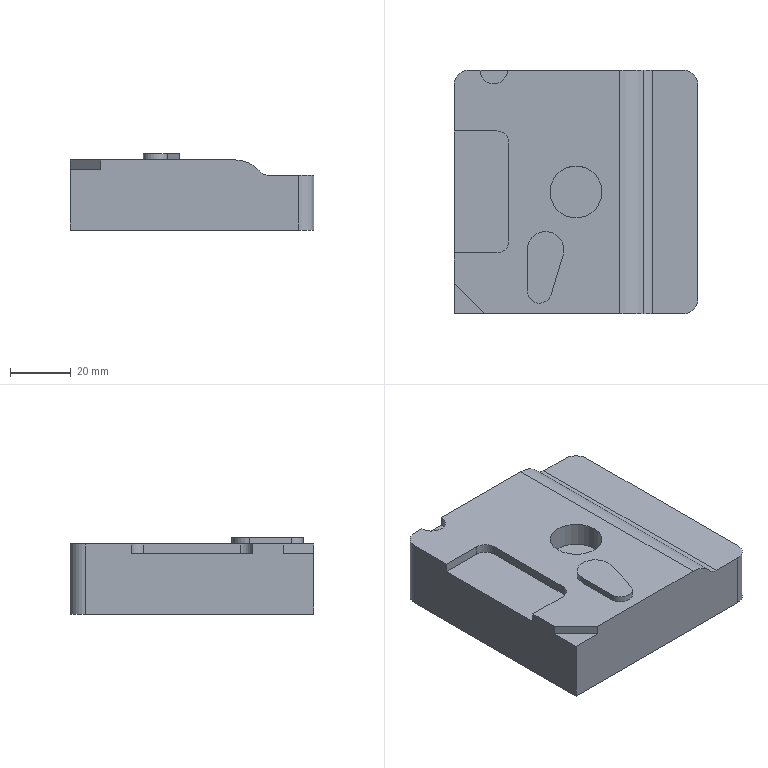NC program | NX | posted with a generic post | part box 80 x 80 x 25 mm
Lines 1871 to 3074 of 8300:
(REST_MILLING , TOOL : D6)
N3740 M6
N3742 G53
N3744 G17 G0 G90 X-22.34 Y-26.538 S0 M3
N3746 G43 Z8. H0
N3748 Z4.717
N3750 G94 G1 Z1.717 F250.
N3752 X-19.3
N3754 Y-19.
N3756 G2 X-1.099 Y-21.696 R-9.3
N3758 G1 X-5.014 Y-34.617
N3760 G2 X-19.3 Y-32.5 R7.3
N3762 G1 Y-26.538
N3764 X-22.34
N3766 Z4.717
N3768 G0 Z8.
N3770 Z4.433
N3772 G1 Z1.433
N3774 X-19.3
N3776 Y-19.
N3778 G2 X-1.099 Y-21.696 R-9.3
N3780 G1 X-5.014 Y-34.617
N3782 G2 X-19.3 Y-32.5 R7.3
N3784 G1 Y-26.538
N3786 X-22.34
N3788 Z4.433
N3790 G0 Z8.
N3792 Z4.15
N3794 G1 Z1.15
N3796 X-19.3
N3798 Y-19.
N3800 G2 X-1.099 Y-21.696 R-9.3
N3802 G1 X-5.014 Y-34.617
N3804 G2 X-19.3 Y-32.5 R7.3
N3806 G1 Y-26.538
N3808 X-22.34
N3810 Z4.15
N3812 G0 Z8.
N3814 Z3.867
N3816 G1 Z0.867
N3818 X-19.3
N3820 Y-19.
N3822 G2 X-1.099 Y-21.696 R-9.3
N3824 G1 X-5.014 Y-34.617
N3826 G2 X-19.3 Y-32.5 R7.3
N3828 G1 Y-26.538
N3830 X-22.34
N3832 Z3.867
N3834 G0 Z8.
N3836 Z3.583
N3838 G1 Z0.583
N3840 X-19.3
N3842 Y-19.
N3844 G2 X-1.099 Y-21.696 R-9.3
N3846 G1 X-5.014 Y-34.617
N3848 G2 X-19.3 Y-32.5 R7.3
N3850 G1 Y-26.538
N3852 X-22.34
N3854 Z3.583
N3856 G0 Z8.
N3858 X-28.365 Y-13.649
N3860 Z3.3
N3862 G1 Z0.3
N3864 X-26.64 Y-16.103
N3866 G3 X-25.34 Y-13.6 R3.06
N3868 G1 Y-13.599
N3870 Y13.6
N3872 G3 X-28.4 Y16.66 R3.06
N3874 G1 X-40.
N3876 G2 X-40.297 Y16.673 R3.34
N3878 G1 Y38.21
N3880 G3 X-41.464 Y40.269 R2.4
N3882 G1 X-41.442 Y40.297
N3884 X-29.53
N3886 G3 X-27.438 Y41.522 R2.4
N3888 X-26.562 Y41.522 R3.06
N3890 X-24.47 Y40.297 R2.4
N3892 G1 X20.731
N3894 G2 X20.761 Y39.88 R3.355
N3896 G1 Y39.854
N3898 Y-39.854
N3900 Y-39.88
N3902 G2 X20.731 Y-40.297 R3.355
N3904 G1 X-31.97
N3906 G3 X-33.695 Y-41.029 R2.4
N3908 G1 X-41.029 Y-33.695
N3910 G3 X-40.297 Y-31.97 R2.4
N3912 G1 Y-16.673
N3914 G2 X-40. Y-16.66 R3.34
N3916 G1 X-28.402
N3918 X-28.4
N3920 G3 X-26.64 Y-16.103 R3.06
N3922 G1 X-22.94 Y-13.601
N3924 Y13.6
N3926 G3 X-28.4 Y19.06 R5.46
N3928 G1 X-37.897
N3930 Y37.897
N3932 X-29.53
N3934 G3 X-27. Y38.618 R4.8
N3936 X-24.47 Y37.897 R4.8
N3938 G1 X18.361
N3940 Y-37.897
N3942 X-6.397
N3944 G3 X-4.554 Y-34.756 R7.78
N3946 G1 X-0.64 Y-21.836
N3948 G3 X-19.78 Y-19. R-9.78
N3950 G1 Y-32.5
N3952 G3 X-17.603 Y-37.897 R7.78
N3954 G1 X-17.258 Y-37.564
N3956 G2 X-19.3 Y-32.5 R7.3
N3958 G1 Y-19.
N3960 G2 X-1.099 Y-21.696 R-9.3
N3962 G1 X-5.014 Y-34.617
N3964 G2 X-17.258 Y-37.564 R7.3
N3966 G1 X-17.603 Y-37.897
N3968 X-31.97
N3970 G3 X-33.256 Y-38.073 R4.8
N3972 G1 X-38.073 Y-33.256
N3974 G3 X-37.897 Y-31.97 R4.8
N3976 G1 Y-19.06
N3978 X-28.402
N3980 G3 X-24.068 Y-16.924 R5.46
N3982 G1 X-22.164 Y-18.385
N3984 G3 X-22.18 Y-19. R12.18
N3986 G1 Y-32.5
N3988 G3 X-21.729 Y-35.497 R10.18
N3990 G1 X-31.97
N3992 G3 X-32.424 Y-35.512 R7.2
N3994 G1 X-35.512 Y-32.424
N3996 G3 X-35.497 Y-31.97 R7.2
N3998 G1 Y-21.46
N4000 X-28.402
N4002 G3 X-22.164 Y-18.385 R7.86
N4004 G1 X-24.58 Y-23.122
N4006 Y-32.5
N4008 G3 X-24.566 Y-33.097 R12.58
N4010 G1 X-31.444
N4012 X-33.097 Y-31.444
N4014 Y-23.86
N4016 X-28.402
N4018 G3 X-24.58 Y-23.122 R10.26
N4020 G1 X-26.98 Y-26.18
N4022 Y-30.697
N4024 X-30.45
N4026 X-30.697 Y-30.45
N4028 Y-26.26
N4030 X-28.402
N4032 G3 X-26.98 Y-26.18 R12.66
N4034 G1 X-24.58 Y-23.122
N4036 X-22.164 Y-18.385
N4038 X-24.068 Y-16.924
N4040 G3 X-22.94 Y-13.601 R5.46
N4042 G1 X-20.54 Y-12.896
N4044 Y13.6
N4046 G3 X-28.4 Y21.46 R7.86
N4048 G1 X-35.497
N4050 Y35.497
N4052 X-29.53
N4054 G3 X-27. Y35.957 R7.2
N4056 X-24.47 Y35.497 R7.2
N4058 G1 X15.961
N4060 Y-35.497
N4062 X-2.271
N4064 X-2.257 Y-35.452
N4066 X-1.333 Y-32.402
N4068 X0.964 Y-33.097
N4070 X3.954 Y-23.227
N4072 G3 X-18.14 Y-6.904 R14.58
N4074 G1 Y13.6
N4076 G3 X-28.4 Y23.86 R10.26
N4078 G1 X-33.097
N4080 Y33.097
N4082 X-29.53
N4084 G3 X-27. Y33.437 R9.6
N4086 X-24.47 Y33.097 R9.6
N4088 G1 X13.561
N4090 Y-33.097
N4092 X0.964
N4094 X4.198 Y-30.697
N4096 X6.251 Y-23.922
N4098 G3 X-0.166 Y-5.157 R16.98
N4100 X-4.157 Y-3.057 R-5.16
N4102 X-15.74 Y-3.02 R16.98
N4104 G1 Y13.6
N4106 G3 X-28.4 Y26.26 R12.66
N4108 G1 X-30.697
N4110 Y30.697
N4112 X-29.53
N4114 G3 X-27. Y30.967 R12.
N4116 X-24.47 Y30.697 R12.
N4118 G1 X11.161
N4120 Y-14.143
N4122 X8.761
N4124 G3 X4.464 Y-6.101 R19.38
N4126 X-7.557 Y0.225 R-7.56
N4128 X-13.34 Y0.09 R19.38
N4130 G1 Y13.6
N4132 G3 X-25.199 Y28.316 R15.06
N4134 X-24.47 Y28.297 R14.4
N4136 G1 X8.761
N4138 Y7.664
N4140 X6.361
N4142 G3 X-9.565 Y2.776 R9.96
N4144 X-10.94 Y2.76 R21.78
N4146 G1 Y13.6
N4148 G3 X-16.005 Y25.897 R17.46
N4150 G1 X6.361
N4152 Y7.664
N4154 X3.961 Y11.708
N4156 G3 X-8.54 Y8.935 R12.36
N4158 G1 Y13.6
N4160 G3 X-11.182 Y23.497 R19.86
N4162 G1 X3.961
N4164 Y11.708
N4166 X1.561 Y14.677
N4168 G3 X-6.14 Y13.422 R14.76
N4170 X-7.441 Y21.097 R22.26
N4172 G1 X1.561
N4174 Y14.677
N4176 X-0.839 Y17.139
N4178 G3 X-3.936 Y16.703 R17.16
N4180 X-4.272 Y18.697 R24.66
N4182 G1 X-0.839
N4184 Y17.139
N4186 X1.561 Y14.677
N4188 X3.961 Y11.708
N4190 X6.361 Y7.664
N4192 X8.761
N4194 Y-14.143
N4196 X11.161
N4198 Y-30.697
N4200 X4.198
N4202 X7.433 Y-28.297
N4204 X8.548 Y-24.618
N4206 G3 X8.761 Y-23.857 R19.38
N4208 G1 Y-28.297
N4210 X7.433
N4212 X0.964 Y-33.097
N4214 X-1.333 Y-32.402
N4216 X1.657 Y-22.531
N4218 G3 X-20.54 Y-12.896 R12.18
N4220 G1 X-19.242 Y-13.648
N4222 X-28.34 Y-13.6
N4224 Z3.3
N4226 G0 Z8.
N4228 X-46.3 Y-27.036
N4230 Z3.
N4232 G1 Z0.
N4234 X-42.697 Y-31.97
N4236 G3 X-42.362 Y-32.362 R3.34
N4238 G1 X-32.362 Y-42.362
N4240 G3 X-31.97 Y-42.697 R3.34
N4242 G1 X-27.036 Y-46.3
N4244 Z3.
N4246 G0 Z8.
N4248 X-26.789
N4250 Z3.
N4252 G1 Z0.
N4254 X-31.901 Y-42.697
N4256 G2 X-32.333 Y-42.333 R3.3
N4258 G1 X-42.333 Y-32.333
N4260 G2 X-42.697 Y-31.901 R3.3
N4262 G1 X-46.3 Y-26.789
N4264 Z3.
N4266 G0 Z8.
N4268 Y-27.036
N4270 Z2.7
N4272 G1 Z-0.3
N4274 X-42.697 Y-31.97
N4276 G3 X-42.362 Y-32.362 R3.34
N4278 G1 X-32.362 Y-42.362
N4280 G3 X-31.97 Y-42.697 R3.34
N4282 G1 X-27.036 Y-46.3
N4284 Z2.7
N4286 G0 Z8.
N4288 X-26.789
N4290 Z2.7
N4292 G1 Z-0.3
N4294 X-31.901 Y-42.697
N4296 G2 X-32.333 Y-42.333 R3.3
N4298 G1 X-42.333 Y-32.333
N4300 G2 X-42.697 Y-31.901 R3.3
N4302 G1 X-46.3 Y-26.789
N4304 Z2.7
N4306 G0 Z8.
N4308 Y-27.036
N4310 Z2.4
N4312 G1 Z-0.6
N4314 X-42.697 Y-31.97
N4316 G3 X-42.362 Y-32.362 R3.34
N4318 G1 X-32.362 Y-42.362
N4320 G3 X-31.97 Y-42.697 R3.34
N4322 G1 X-27.036 Y-46.3
N4324 Z2.4
N4326 G0 Z8.
N4328 X-26.789
N4330 Z2.4
N4332 G1 Z-0.6
N4334 X-31.901 Y-42.697
N4336 G2 X-32.333 Y-42.333 R3.3
N4338 G1 X-42.333 Y-32.333
N4340 G2 X-42.697 Y-31.901 R3.3
N4342 G1 X-46.3 Y-26.789
N4344 Z2.4
N4346 G0 Z8.
N4348 Y-27.035
N4350 Z2.1
N4352 G1 Z-0.9
N4354 X-42.698 Y-31.97
N4356 G3 X-42.362 Y-32.362 R3.34
N4358 G1 X-32.363 Y-42.361
N4360 X-32.362 Y-42.362
N4362 G3 X-31.97 Y-42.698 R3.34
N4364 G1 X-27.035 Y-46.3
N4366 Z2.1
N4368 G0 Z8.
N4370 X-26.789
N4372 Z2.1
N4374 G1 Z-0.9
N4376 X-31.901 Y-42.698
N4378 G2 X-32.333 Y-42.333 R3.3
N4380 G1 X-42.333 Y-32.333
N4382 G2 X-42.698 Y-31.901 R3.3
N4384 G1 X-46.3 Y-26.789
N4386 Z2.1
N4388 G0 Z8.
N4390 Y-27.035
N4392 Z1.8
N4394 G1 Z-1.2
N4396 X-42.698 Y-31.969
N4398 G3 X-42.362 Y-32.362 R3.34
N4400 G1 X-32.363 Y-42.361
N4402 X-32.362 Y-42.362
N4404 G3 X-31.969 Y-42.698 R3.34
N4406 G1 X-27.035 Y-46.3
N4408 Z1.8
N4410 G0 Z8.
N4412 X-26.788
N4414 Z1.8
N4416 G1 Z-1.2
N4418 X-31.901 Y-42.698
N4420 G2 X-32.333 Y-42.333 R3.3
N4422 G1 X-42.333 Y-32.333
N4424 G2 X-42.698 Y-31.901 R3.3
N4426 G1 X-46.3 Y-26.788
N4428 Z1.8
N4430 G0 Z8.
N4432 Y-27.035
N4434 Z1.5
N4436 G1 Z-1.5
N4438 X-42.698 Y-31.969
N4440 G3 X-42.362 Y-32.362 R3.34
N4442 G1 X-32.363 Y-42.361
N4444 X-32.362 Y-42.362
N4446 G3 X-31.969 Y-42.698 R3.34
N4448 G1 X-27.035 Y-46.3
N4450 Z1.5
N4452 G0 Z8.
N4454 X-26.788
N4456 Z1.5
N4458 G1 Z-1.5
N4460 X-31.901 Y-42.698
N4462 G2 X-32.333 Y-42.333 R3.3
N4464 G1 X-42.333 Y-32.333
N4466 G2 X-42.698 Y-31.901 R3.3
N4468 G1 X-46.3 Y-26.788
N4470 Z1.5
N4472 G0 Z8.
N4474 Y-27.035
N4476 Z1.2
N4478 G1 Z-1.8
N4480 X-42.698 Y-31.969
N4482 G3 X-42.362 Y-32.362 R3.34
N4484 G1 X-32.363 Y-42.361
N4486 X-32.362 Y-42.362
N4488 G3 X-31.969 Y-42.698 R3.34
N4490 G1 X-27.035 Y-46.3
N4492 Z1.2
N4494 G0 Z8.
N4496 X-26.788
N4498 Z1.2
N4500 G1 Z-1.8
N4502 X-31.901 Y-42.698
N4504 G2 X-32.333 Y-42.333 R3.3
N4506 G1 X-42.333 Y-32.333
N4508 G2 X-42.698 Y-31.901 R3.3
N4510 G1 X-46.3 Y-26.788
N4512 Z1.2
N4514 G0 Z8.
N4516 Y-27.035
N4518 Z0.9
N4520 G1 Z-2.1
N4522 X-42.698 Y-31.969
N4524 G3 X-42.362 Y-32.362 R3.34
N4526 G1 X-32.363 Y-42.361
N4528 X-32.362 Y-42.362
N4530 X-32.359 Y-42.365
N4532 G3 X-31.969 Y-42.698 R3.34
N4534 G1 X-27.035 Y-46.3
N4536 Z0.9
N4538 G0 Z8.
N4540 X-26.788
N4542 Z0.9
N4544 G1 Z-2.1
N4546 X-31.901 Y-42.698
N4548 G2 X-32.333 Y-42.333 R3.3
N4550 G1 X-42.333 Y-32.333
N4552 G2 X-42.698 Y-31.901 R3.3
N4554 G1 X-46.3 Y-26.788
N4556 Z0.9
N4558 G0 Z8.
N4560 Y-27.035
N4562 Z0.6
N4564 G1 Z-2.4
N4566 X-42.698 Y-31.969
N4568 G3 X-42.362 Y-32.362 R3.34
N4570 G1 X-32.363 Y-42.361
N4572 X-32.362 Y-42.362
N4574 X-32.359 Y-42.365
N4576 G3 X-31.969 Y-42.698 R3.34
N4578 G1 X-27.035 Y-46.3
N4580 Z0.6
N4582 G0 Z8.
N4584 X-26.788
N4586 Z0.6
N4588 G1 Z-2.4
N4590 X-31.901 Y-42.698
N4592 G2 X-32.333 Y-42.333 R3.3
N4594 G1 X-42.333 Y-32.333
N4596 G2 X-42.698 Y-31.901 R3.3
N4598 G1 X-46.3 Y-26.788
N4600 Z0.6
N4602 G0 Z8.
N4604 X-26.788 Y-46.3
N4606 Z0.3
N4608 G1 Z-2.7
N4610 X-31.901 Y-42.698
N4612 G2 X-32.333 Y-42.333 R3.3
N4614 G1 X-42.333 Y-32.333
N4616 G2 X-42.698 Y-31.901 R3.3
N4618 G1 X-46.3 Y-26.788
N4620 Z0.3
N4622 G0 Z8.
N4624 X-38.837 Y-45.698
N4626 Z0.3
N4628 G1 Z-2.7
N4630 Y-40.298
N4632 X-39.774
N4634 X-39.91 Y-40.312
N4636 G2 X-40.312 Y-39.91 R0.367
N4638 G1 X-40.298 Y-39.774
N4640 Y-37.763
N4642 X-37.763 Y-40.298
N4644 X-38.837
N4646 Y-45.698
N4648 Z0.3
N4650 G0 Z8.
N4652 X-46.3 Y22.964
N4654 Z3.
N4656 G1 Z0.
N4658 X-42.697 Y18.03
N4660 G3 X-40. Y16.66 R3.34
N4662 G1 X-28.4
N4664 G2 X-25.34 Y13.6 R3.06
N4666 G1 Y-13.599
N4668 Y-13.6
N4670 G2 X-28.4 Y-16.66 R3.06
N4672 G1 X-28.402
N4674 X-40.
N4676 G3 X-42.697 Y-18.03 R3.34
N4678 G1 X-46.3 Y-22.964
N4680 Z3.
N4682 G0 Z8.
N4684 Y-23.211
N4686 Z3.
N4688 G1 Z0.
N4690 X-42.697 Y-18.099
N4692 G2 X-40. Y-16.7 R3.3
N4694 G1 X-26.
N4696 G3 X-25.3 Y-16. R0.7
N4698 G1 Y16.
N4700 G3 X-26. Y16.7 R0.7
N4702 G1 X-40.
N4704 G2 X-42.697 Y18.099 R3.3
N4706 G1 X-46.3 Y23.211
N4708 Z3.
N4710 G0 Z8.
N4712 Y22.964
N4714 Z2.7
N4716 G1 Z-0.3
N4718 X-42.697 Y18.03
N4720 G3 X-40. Y16.66 R3.34
N4722 G1 X-28.4
N4724 G2 X-25.34 Y13.6 R3.06
N4726 G1 Y-13.599
N4728 Y-13.6
N4730 G2 X-28.4 Y-16.66 R3.06
N4732 G1 X-28.402
N4734 X-40.
N4736 G3 X-42.697 Y-18.03 R3.34
N4738 G1 X-46.3 Y-22.964
N4740 Z2.7
N4742 G0 Z8.
N4744 Y-23.211
N4746 Z2.7
N4748 G1 Z-0.3
N4750 X-42.697 Y-18.099
N4752 G2 X-40. Y-16.7 R3.3
N4754 G1 X-26.
N4756 G3 X-25.3 Y-16. R0.7
N4758 G1 Y16.
N4760 G3 X-26. Y16.7 R0.7
N4762 G1 X-40.
N4764 G2 X-42.697 Y18.099 R3.3
N4766 G1 X-46.3 Y23.211
N4768 Z2.7
N4770 G0 Z8.
N4772 Y22.964
N4774 Z2.4
N4776 G1 Z-0.6
N4778 X-42.697 Y18.03
N4780 G3 X-40. Y16.66 R3.34
N4782 G1 X-28.4
N4784 G2 X-25.34 Y13.6 R3.06
N4786 G1 Y-13.599
N4788 Y-13.6
N4790 G2 X-28.4 Y-16.66 R3.06
N4792 G1 X-28.402
N4794 X-40.
N4796 G3 X-42.697 Y-18.03 R3.34
N4798 G1 X-46.3 Y-22.964
N4800 Z2.4
N4802 G0 Z8.
N4804 Y-23.211
N4806 Z2.4
N4808 G1 Z-0.6
N4810 X-42.697 Y-18.099
N4812 G2 X-40. Y-16.7 R3.3
N4814 G1 X-26.
N4816 G3 X-25.3 Y-16. R0.7
N4818 G1 Y16.
N4820 G3 X-26. Y16.7 R0.7
N4822 G1 X-40.
N4824 G2 X-42.697 Y18.099 R3.3
N4826 G1 X-46.3 Y23.211
N4828 Z2.4
N4830 G0 Z8.
N4832 Y22.965
N4834 Z2.1
N4836 G1 Z-0.9
N4838 X-42.698 Y18.03
N4840 G3 X-40. Y16.66 R3.34
N4842 G1 X-28.4
N4844 G2 X-25.34 Y13.6 R3.06
N4846 G1 Y-13.599
N4848 Y-13.6
N4850 G2 X-28.4 Y-16.66 R3.06
N4852 G1 X-28.402
N4854 X-40.
N4856 G3 X-42.698 Y-18.03 R3.34
N4858 G1 X-46.3 Y-22.965
N4860 Z2.1
N4862 G0 Z8.
N4864 Y-23.211
N4866 Z2.1
N4868 G1 Z-0.9
N4870 X-42.698 Y-18.099
N4872 G2 X-40. Y-16.7 R3.3
N4874 G1 X-26.
N4876 G3 X-25.3 Y-16. R0.7
N4878 G1 Y16.
N4880 G3 X-26. Y16.7 R0.7
N4882 G1 X-40.
N4884 G2 X-42.698 Y18.099 R3.3
N4886 G1 X-46.3 Y23.211
N4888 Z2.1
N4890 G0 Z8.
N4892 Y22.965
N4894 Z1.8
N4896 G1 Z-1.2
N4898 X-42.698 Y18.031
N4900 G3 X-40. Y16.66 R3.34
N4902 G1 X-28.4
N4904 G2 X-25.34 Y13.6 R3.06
N4906 G1 Y-13.599
N4908 Y-13.6
N4910 G2 X-28.4 Y-16.66 R3.06
N4912 G1 X-28.402
N4914 X-40.
N4916 G3 X-42.698 Y-18.031 R3.34
N4918 G1 X-46.3 Y-22.965
N4920 Z1.8
N4922 G0 Z8.
N4924 Y-23.212
N4926 Z1.8
N4928 G1 Z-1.2
N4930 X-42.698 Y-18.099
N4932 G2 X-40. Y-16.7 R3.3
N4934 G1 X-26.
N4936 G3 X-25.3 Y-16. R0.7
N4938 G1 Y16.
N4940 G3 X-26. Y16.7 R0.7
N4942 G1 X-40.
N4944 G2 X-42.698 Y18.099 R3.3
N4946 G1 X-46.3 Y23.212
N4948 Z1.8
N4950 G0 Z8.
N4952 Y22.965
N4954 Z1.5
N4956 G1 Z-1.5
N4958 X-42.698 Y18.031
N4960 G3 X-40. Y16.66 R3.34
N4962 G1 X-28.4
N4964 G2 X-25.34 Y13.6 R3.06
N4966 G1 Y-13.599
N4968 Y-13.6
N4970 G2 X-28.4 Y-16.66 R3.06
N4972 G1 X-28.402
N4974 X-40.
N4976 G3 X-42.698 Y-18.031 R3.34
N4978 G1 X-46.3 Y-22.965
N4980 Z1.5
N4982 G0 Z8.
N4984 Y-23.212
N4986 Z1.5
N4988 G1 Z-1.5
N4990 X-42.698 Y-18.099
N4992 G2 X-40. Y-16.7 R3.3
N4994 G1 X-26.
N4996 G3 X-25.3 Y-16. R0.7
N4998 G1 Y16.
N5000 G3 X-26. Y16.7 R0.7
N5002 G1 X-40.
N5004 G2 X-42.698 Y18.099 R3.3
N5006 G1 X-46.3 Y23.212
N5008 Z1.5
N5010 G0 Z8.
N5012 Y22.965
N5014 Z1.2
N5016 G1 Z-1.8
N5018 X-42.698 Y18.031
N5020 G3 X-40. Y16.66 R3.34
N5022 G1 X-28.4
N5024 G2 X-25.34 Y13.6 R3.06
N5026 G1 Y-13.599
N5028 Y-13.6
N5030 G2 X-28.4 Y-16.66 R3.06
N5032 G1 X-28.402
N5034 X-40.
N5036 G3 X-42.698 Y-18.031 R3.34
N5038 G1 X-46.3 Y-22.965
N5040 Z1.2
N5042 G0 Z8.
N5044 Y-23.212
N5046 Z1.2
N5048 G1 Z-1.8
N5050 X-42.698 Y-18.099
N5052 G2 X-40. Y-16.7 R3.3
N5054 G1 X-26.
N5056 G3 X-25.3 Y-16. R0.7
N5058 G1 Y16.
N5060 G3 X-26. Y16.7 R0.7
N5062 G1 X-40.
N5064 G2 X-42.698 Y18.099 R3.3
N5066 G1 X-46.3 Y23.212
N5068 Z1.2
N5070 G0 Z8.
N5072 Y22.965
N5074 Z0.9
N5076 G1 Z-2.1
N5078 X-42.698 Y18.031
N5080 G3 X-40. Y16.66 R3.34
N5082 G1 X-28.4
N5084 G2 X-25.34 Y13.6 R3.06
N5086 G1 Y-13.599
N5088 Y-13.6
N5090 G2 X-28.4 Y-16.66 R3.06
N5092 G1 X-28.402
N5094 X-40.
N5096 G3 X-42.698 Y-18.031 R3.34
N5098 G1 X-46.3 Y-22.965
N5100 Z0.9
N5102 G0 Z8.
N5104 Y-23.212
N5106 Z0.9
N5108 G1 Z-2.1
N5110 X-42.698 Y-18.099
N5112 G2 X-40. Y-16.7 R3.3
N5114 G1 X-26.
N5116 G3 X-25.3 Y-16. R0.7
N5118 G1 Y16.
N5120 G3 X-26. Y16.7 R0.7
N5122 G1 X-40.
N5124 G2 X-42.698 Y18.099 R3.3
N5126 G1 X-46.3 Y23.212
N5128 Z0.9
N5130 G0 Z8.
N5132 Y22.965
N5134 Z0.6
N5136 G1 Z-2.4
N5138 X-42.698 Y18.031
N5140 G3 X-40. Y16.66 R3.34
N5142 G1 X-28.4
N5144 G2 X-25.34 Y13.6 R3.06
N5146 G1 Y-13.599
N5148 Y-13.6
N5150 G2 X-28.4 Y-16.66 R3.06
N5152 G1 X-28.402
N5154 X-40.
N5156 G3 X-42.698 Y-18.031 R3.34
N5158 G1 X-46.3 Y-22.965
N5160 Z0.6
N5162 G0 Z8.
N5164 Y-23.212
N5166 Z0.6
N5168 G1 Z-2.4
N5170 X-42.698 Y-18.099
N5172 G2 X-40. Y-16.7 R3.3
N5174 G1 X-26.
N5176 G3 X-25.3 Y-16. R0.7
N5178 G1 Y16.
N5180 G3 X-26. Y16.7 R0.7
N5182 G1 X-40.
N5184 G2 X-42.698 Y18.099 R3.3
N5186 G1 X-46.3 Y23.212
N5188 Z0.6
N5190 G0 Z8.
N5192 Y-23.212
N5194 Z0.3
N5196 G1 Z-2.7
N5198 X-42.698 Y-18.099
N5200 G2 X-40. Y-16.7 R3.3
N5202 G1 X-26.
N5204 G3 X-25.3 Y-16. R0.7
N5206 G1 Y16.
N5208 G3 X-26. Y16.7 R0.7
N5210 G1 X-40.
N5212 G2 X-42.698 Y18.099 R3.3
N5214 G1 X-46.3 Y23.212
N5216 Z0.3
N5218 G0 Z8.
N5220 X-45.698 Y0.
N5222 Z0.3
N5224 G1 Z-2.7
N5226 X-40.298
N5228 Y14.308
N5230 G3 X-40. Y14.3 R5.7
N5232 G1 X-27.7
N5234 Y-14.3
N5236 X-40.
N5238 G3 X-40.298 Y-14.308 R5.7
N5240 G1 Y0.
N5242 X-37.898
N5244 Y11.9
N5246 X-30.1
N5248 Y-11.9
N5250 X-37.898
N5252 Y0.
N5254 X-35.498
N5256 Y9.5
N5258 X-32.5
N5260 Y-9.5
N5262 X-35.498
N5264 Y0.
N5266 X-40.298
N5268 X-45.698
N5270 Z0.3
N5272 G0 Z8.
N5274 X-30.004 Y46.12
N5276 Z3.
N5278 G1 Z0.
N5280 X-38.21 Y42.697
N5282 G3 X-42.697 Y38.21 R8.34
N5284 G1 X-43.852 Y35.441
N5286 X-46.286 Y35.563
N5288 Z3.
N5290 G0 Z8.
N5292 X-46.292 Y35.413
N5294 Z3.
N5296 G1 Z0.
N5298 X-43.82 Y35.323
N5300 X-42.697 Y38.105
N5302 G2 X-38.105 Y42.697 R8.3
N5304 G1 X-29.772 Y46.058
N5306 Z3.
N5308 G0 Z8.
N5310 X-30.004 Y46.12
N5312 Z2.7
N5314 G1 Z-0.3
N5316 X-38.21 Y42.697
N5318 G3 X-42.697 Y38.21 R8.34
N5320 G1 X-43.852 Y35.441
N5322 X-46.286 Y35.563
N5324 Z2.7
N5326 G0 Z8.
N5328 X-46.292 Y35.413
N5330 Z2.7
N5332 G1 Z-0.3
N5334 X-43.82 Y35.322
N5336 X-42.697 Y38.105
N5338 G2 X-38.105 Y42.697 R8.3
N5340 G1 X-29.772 Y46.058
N5342 Z2.7
N5344 G0 Z8.
N5346 X-30.004 Y46.12
N5348 Z2.4
N5350 G1 Z-0.6
N5352 X-38.21 Y42.697
N5354 G3 X-42.697 Y38.21 R8.34
N5356 G1 X-43.852 Y35.441
N5358 X-46.286 Y35.562
N5360 Z2.4
N5362 G0 Z8.
N5364 X-46.292 Y35.413
N5366 Z2.4
N5368 G1 Z-0.6
N5370 X-43.82 Y35.322
N5372 X-42.697 Y38.105
N5374 G2 X-38.105 Y42.697 R8.3
N5376 G1 X-29.772 Y46.058
N5378 Z2.4
N5380 G0 Z8.
N5382 X-30.004 Y46.12
N5384 Z2.1
N5386 G1 Z-0.9
N5388 X-38.21 Y42.698
N5390 G3 X-42.698 Y38.21 R8.34
N5392 G1 X-43.852 Y35.441
N5394 X-46.286 Y35.562
N5396 Z2.1
N5398 G0 Z8.
N5400 X-46.292 Y35.413
N5402 Z2.1
N5404 G1 Z-0.9
N5406 X-43.82 Y35.322
N5408 X-42.698 Y38.105
N5410 G2 X-38.105 Y42.698 R8.3
N5412 G1 X-29.772 Y46.058
N5414 Z2.1
N5416 G0 Z8.
N5418 X-30.003 Y46.12
N5420 Z1.8
N5422 G1 Z-1.2
N5424 X-38.21 Y42.698
N5426 G3 X-42.698 Y38.21 R8.34
N5428 G1 X-43.852 Y35.441
N5430 X-46.286 Y35.562
N5432 Z1.8
N5434 G0 Z8.
N5436 X-46.292 Y35.413
N5438 Z1.8
N5440 G1 Z-1.2
N5442 X-43.82 Y35.322
N5444 X-42.698 Y38.104
N5446 G2 X-38.104 Y42.698 R8.3
N5448 G1 X-29.772 Y46.058
N5450 Z1.8
N5452 G0 Z8.
N5454 X-30.003 Y46.12
N5456 Z1.5
N5458 G1 Z-1.5
N5460 X-38.21 Y42.698
N5462 G3 X-42.698 Y38.21 R8.34
N5464 G1 X-43.852 Y35.441
N5466 X-46.286 Y35.562
N5468 Z1.5
N5470 G0 Z8.
N5472 X-46.292 Y35.412
N5474 Z1.5
N5476 G1 Z-1.5
N5478 X-43.82 Y35.322
N5480 X-42.698 Y38.104
N5482 G2 X-38.104 Y42.698 R8.3
N5484 G1 X-29.771 Y46.058
N5486 Z1.5
N5488 G0 Z8.
N5490 X-30.003 Y46.12
N5492 Z1.2
N5494 G1 Z-1.8
N5496 X-38.21 Y42.698
N5498 G3 X-42.698 Y38.21 R8.34
N5500 G1 X-43.852 Y35.441
N5502 X-46.286 Y35.562
N5504 Z1.2
N5506 G0 Z8.
N5508 X-46.292 Y35.412
N5510 Z1.2
N5512 G1 Z-1.8
N5514 X-43.82 Y35.322
N5516 X-42.698 Y38.104
N5518 G2 X-38.104 Y42.698 R8.3
N5520 G1 X-29.771 Y46.058
N5522 Z1.2
N5524 G0 Z8.
N5526 X-30.003 Y46.12
N5528 Z0.9
N5530 G1 Z-2.1
N5532 X-38.21 Y42.698
N5534 G3 X-42.698 Y38.21 R8.34
N5536 G1 X-43.852 Y35.441
N5538 X-46.286 Y35.562
N5540 Z0.9
N5542 G0 Z8.
N5544 X-46.292 Y35.412
N5546 Z0.9
N5548 G1 Z-2.1
N5550 X-43.82 Y35.322
N5552 X-42.698 Y38.104
N5554 G2 X-38.104 Y42.698 R8.3
N5556 G1 X-29.771 Y46.058
N5558 Z0.9
N5560 G0 Z8.
N5562 X-30.003 Y46.119
N5564 Z0.6
N5566 G1 Z-2.4
N5568 X-38.21 Y42.698
N5570 G3 X-42.698 Y38.21 R8.34
N5572 G1 X-43.852 Y35.441
N5574 X-46.286 Y35.562
N5576 Z0.6
N5578 G0 Z8.
N5580 X-46.292 Y35.412
N5582 Z0.6
N5584 G1 Z-2.4
N5586 X-43.82 Y35.322
N5588 X-42.698 Y38.104
N5590 G2 X-38.104 Y42.698 R8.3
N5592 G1 X-29.771 Y46.058
N5594 Z0.6
N5596 G0 Z8.
N5598 X-30.003 Y46.119
N5600 Z0.3
N5602 G1 Z-2.7
N5604 X-38.209 Y42.698
N5606 G3 X-42.698 Y38.209 R8.34
N5608 G1 X-43.852 Y35.44
N5610 X-46.286 Y35.562
N5612 Z0.3
N5614 G0 Z8.
N5616 X-46.292 Y35.412
N5618 Z0.3
N5620 G1 Z-2.7
N5622 X-43.82 Y35.322
N5624 X-42.698 Y38.104
N5626 G2 X-38.104 Y42.698 R8.3
N5628 G1 X-29.771 Y46.058
N5630 Z0.3
N5632 G0 Z8.
N5634 X-35.561 Y46.286
N5636 Z0.014
N5638 G1 Z-2.986
N5640 X-35.44 Y43.852
N5642 X-38.209 Y42.698
N5644 G3 X-42.698 Y38.209 R8.34
N5646 G1 X-43.852 Y35.44
N5648 X-46.286 Y35.561
N5650 Z0.014
N5652 G0 Z8.
N5654 X-46.292 Y35.412
N5656 Z0.014
N5658 G1 Z-2.986
N5660 X-43.82 Y35.322
N5662 X-42.698 Y38.104
N5664 G2 X-38.104 Y42.698 R8.3
N5666 G1 X-35.322 Y43.82
N5668 X-35.412 Y46.292
N5670 Z0.014
N5672 G0 Z8.
N5674 X-35.561 Y46.286
N5676 Z-0.271
N5678 G1 Z-3.271
N5680 X-35.44 Y43.852
N5682 X-38.209 Y42.698
N5684 G3 X-42.698 Y38.209 R8.34
N5686 G1 X-43.852 Y35.44
N5688 X-46.286 Y35.561
N5690 Z-0.271
N5692 G0 Z8.
N5694 X-46.292 Y35.412
N5696 Z-0.271
N5698 G1 Z-3.271
N5700 X-43.82 Y35.322
N5702 X-42.698 Y38.104
N5704 G2 X-38.104 Y42.698 R8.3
N5706 G1 X-35.322 Y43.82
N5708 X-35.412 Y46.292
N5710 Z-0.271
N5712 G0 Z8.
N5714 X-35.561 Y46.286
N5716 Z-0.557
N5718 G1 Z-3.557
N5720 X-35.44 Y43.852
N5722 X-38.209 Y42.698
N5724 G3 X-42.698 Y38.209 R8.34
N5726 G1 X-43.852 Y35.44
N5728 X-46.286 Y35.561
N5730 Z-0.557
N5732 G0 Z8.
N5734 X-46.293 Y35.412
N5736 Z-0.557
N5738 G1 Z-3.557
N5740 X-43.82 Y35.321
N5742 X-42.698 Y38.104
N5744 G2 X-38.104 Y42.698 R8.3
N5746 G1 X-35.321 Y43.82
N5748 X-35.412 Y46.293
N5750 Z-0.557
N5752 G0 Z8.
N5754 X-35.561 Y46.286
N5756 Z-0.843
N5758 G1 Z-3.843
N5760 X-35.44 Y43.852
N5762 X-38.209 Y42.698
N5764 G3 X-42.698 Y38.209 R8.34
N5766 G1 X-43.852 Y35.44
N5768 X-46.286 Y35.561
N5770 Z-0.843
N5772 G0 Z8.
N5774 X-46.293 Y35.411
N5776 Z-0.843
N5778 G1 Z-3.843
N5780 X-43.82 Y35.321
N5782 X-42.698 Y38.104
N5784 G2 X-38.104 Y42.698 R8.3
N5786 G1 X-35.321 Y43.82
N5788 X-35.411 Y46.293
N5790 Z-0.843
N5792 G0 Z8.
N5794 X-35.561 Y46.286
N5796 Z-1.129
N5798 G1 Z-4.129
N5800 X-35.44 Y43.852
N5802 X-38.209 Y42.698
N5804 G3 X-42.698 Y38.209 R8.34
N5806 G1 X-43.852 Y35.44
N5808 X-46.286 Y35.561
N5810 Z-1.129
N5812 G0 Z8.
N5814 X-46.293 Y35.411
N5816 Z-1.129
N5818 G1 Z-4.129
N5820 X-43.82 Y35.321
N5822 X-42.698 Y38.104
N5824 G2 X-38.104 Y42.698 R8.3
N5826 G1 X-35.321 Y43.82
N5828 X-35.411 Y46.293
N5830 Z-1.129
N5832 G0 Z8.
N5834 X-35.561 Y46.286
N5836 Z-1.414
N5838 G1 Z-4.414
N5840 X-35.44 Y43.852
N5842 X-38.209 Y42.698
N5844 G3 X-42.698 Y38.209 R8.34
N5846 G1 X-43.852 Y35.44
N5848 X-46.286 Y35.561
N5850 Z-1.414
N5852 G0 Z8.
N5854 X-46.293 Y35.411
N5856 Z-1.414
N5858 G1 Z-4.414
N5860 X-43.82 Y35.321
N5862 X-42.698 Y38.104
N5864 G2 X-38.104 Y42.698 R8.3
N5866 G1 X-35.321 Y43.82
N5868 X-35.411 Y46.293
N5870 Z-1.414
N5872 G0 Z8.
N5874 X-35.561 Y46.286
N5876 Z-1.7
N5878 G1 Z-4.7
N5880 X-35.44 Y43.852
N5882 X-38.209 Y42.698
N5884 G3 X-42.698 Y38.209 R8.34
N5886 G1 X-43.852 Y35.44
N5888 X-46.286 Y35.561
N5890 Z-1.7
N5892 G0 Z8.
N5894 X-46.293 Y35.411
N5896 Z-1.7
N5898 G1 Z-4.7
N5900 X-43.82 Y35.321
N5902 X-42.698 Y38.103
N5904 G2 X-38.103 Y42.698 R8.3
N5906 G1 X-35.321 Y43.82
N5908 X-35.411 Y46.293
N5910 Z-1.7
N5912 G0 Z8.
N5914 X-35.561 Y46.286
N5916 Z-2.
N5918 G1 Z-5.
N5920 X-35.44 Y43.852
N5922 X-38.209 Y42.698
N5924 G3 X-42.698 Y38.209 R8.34
N5926 G1 X-43.852 Y35.44
N5928 X-46.286 Y35.561
N5930 Z-2.
N5932 G0 Z8.
N5934 X-46.293 Y35.411
N5936 Z-2.
N5938 G1 Z-5.
N5940 X-43.82 Y35.321
N5942 X-42.698 Y38.103
N5944 G2 X-38.103 Y42.698 R8.3
N5946 G1 X-35.321 Y43.82
N5948 X-35.411 Y46.293
N5950 Z-2.
N5952 G0 Z8.
N5954 X-35.561 Y46.286
N5956 Z-2.3
N5958 G1 Z-5.3
N5960 X-35.44 Y43.852
N5962 X-38.209 Y42.698
N5964 G3 X-42.698 Y38.209 R8.34
N5966 G1 X-43.852 Y35.44
N5968 X-46.286 Y35.561
N5970 Z-2.3
N5972 G0 Z8.
N5974 X-46.293 Y35.411
N5976 Z-2.3
N5978 G1 Z-5.3
N5980 X-43.82 Y35.321
N5982 X-42.698 Y38.103
N5984 G2 X-38.103 Y42.698 R8.3
N5986 G1 X-35.321 Y43.82
N5988 X-35.411 Y46.293
N5990 Z-2.3
N5992 G0 Z8.
N5994 X-35.56 Y46.286
N5996 Z-2.6
N5998 G1 Z-5.6
N6000 X-35.44 Y43.852
N6002 X-38.209 Y42.698
N6004 G3 X-42.698 Y38.209 R8.34
N6006 G1 X-43.852 Y35.44
N6008 X-46.286 Y35.56
N6010 Z-2.6
N6012 G0 Z8.
N6014 X-46.293 Y35.411
N6016 Z-2.6
N6018 G1 Z-5.6
N6020 X-43.82 Y35.321
N6022 X-42.698 Y38.103
N6024 G2 X-38.103 Y42.698 R8.3
N6026 G1 X-35.321 Y43.82
N6028 X-35.411 Y46.293
N6030 Z-2.6
N6032 G0 Z8.
N6034 X-35.56 Y46.286
N6036 Z-2.9
N6038 G1 Z-5.9
N6040 X-35.44 Y43.852
N6042 X-38.209 Y42.698
N6044 G3 X-42.698 Y38.209 R8.34
N6046 G1 X-43.852 Y35.44
N6048 X-46.286 Y35.56
N6050 Z-2.9
N6052 G0 Z8.
N6054 X-46.293 Y35.411
N6056 Z-2.9
N6058 G1 Z-5.9
N6060 X-43.82 Y35.321
N6062 X-42.698 Y38.103
N6064 G2 X-38.103 Y42.698 R8.3
N6066 G1 X-35.321 Y43.82
N6068 X-35.411 Y46.293
N6070 Z-2.9
N6072 G0 Z8.
N6074 X-35.56 Y46.286
N6076 Z-3.2
N6078 G1 Z-6.2
N6080 X-35.439 Y43.852
N6082 X-38.209 Y42.698
N6084 G3 X-42.698 Y38.209 R8.34
N6086 G1 X-43.852 Y35.439
N6088 X-46.286 Y35.56
N6090 Z-3.2
N6092 G0 Z8.
N6094 X-46.293 Y35.411
N6096 Z-3.2
N6098 G1 Z-6.2
N6100 X-43.82 Y35.321
N6102 X-42.698 Y38.103
N6104 G2 X-38.103 Y42.698 R8.3
N6106 G1 X-35.321 Y43.82
N6108 X-35.411 Y46.293
N6110 Z-3.2
N6112 G0 Z8.
N6114 X-35.56 Y46.286
N6116 Z-3.5
N6118 G1 Z-6.5
N6120 X-35.439 Y43.852
N6122 X-38.208 Y42.698
N6124 G3 X-42.698 Y38.208 R8.34
N6126 G1 X-43.852 Y35.439
N6128 X-46.286 Y35.56
N6130 Z-3.5
N6132 G0 Z8.
N6134 X-46.293 Y35.41
N6136 Z-3.5
N6138 G1 Z-6.5
N6140 X-43.82 Y35.321